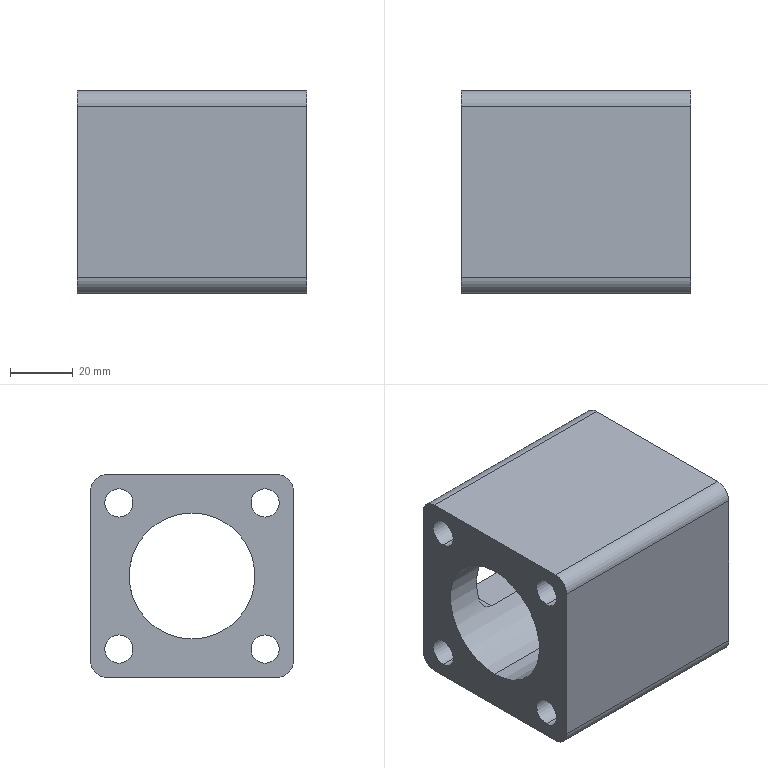Part | STEP file | 1 solid | 81 faces | box 73 x 64.5 x 64.5 mm | volume 159497 mm3 | cylinder 48 | plane 19 | cone 14 | commonest cylinder face diameters 2.5 x8 4.2 x8 8 x8 9 x8 14 x8 10 x4